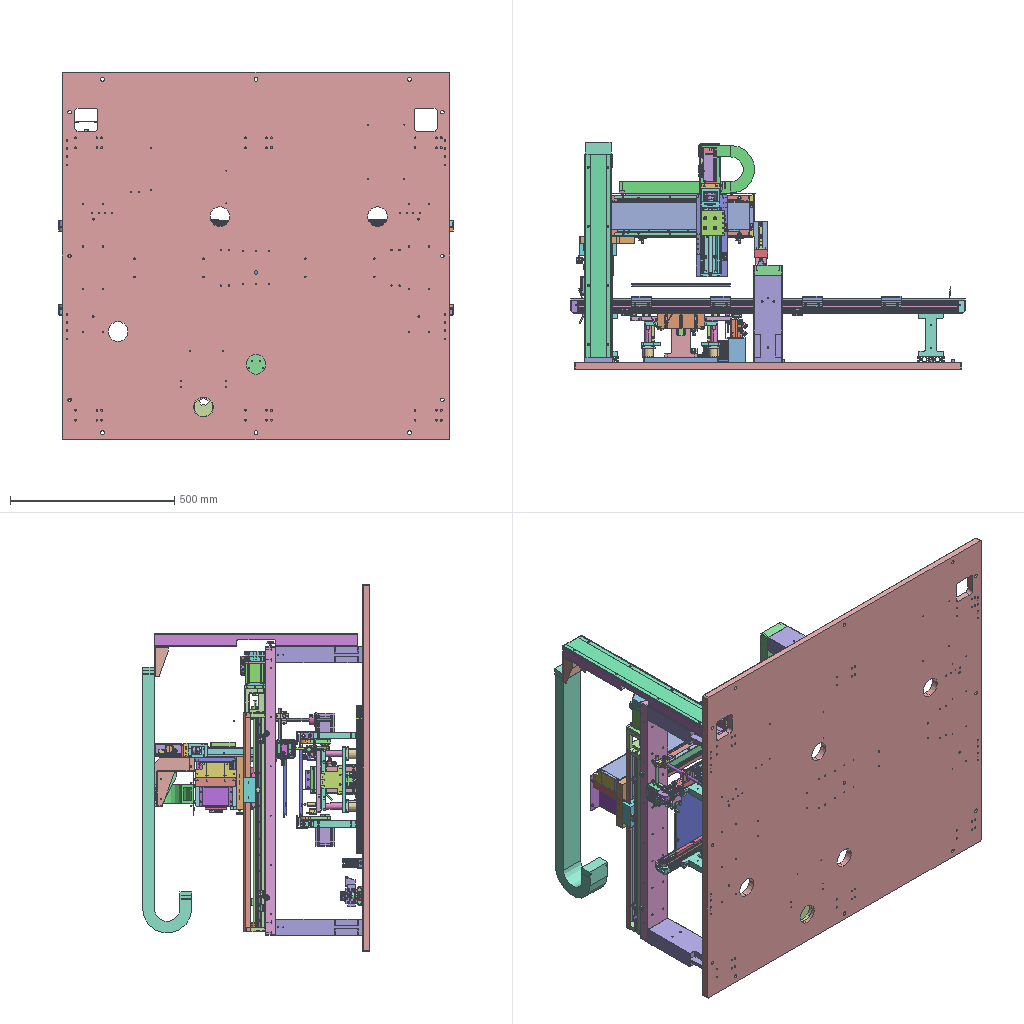Assembly | STEP file | 141 different items | 353 placed | box 1201 x 691 x 1120 mm
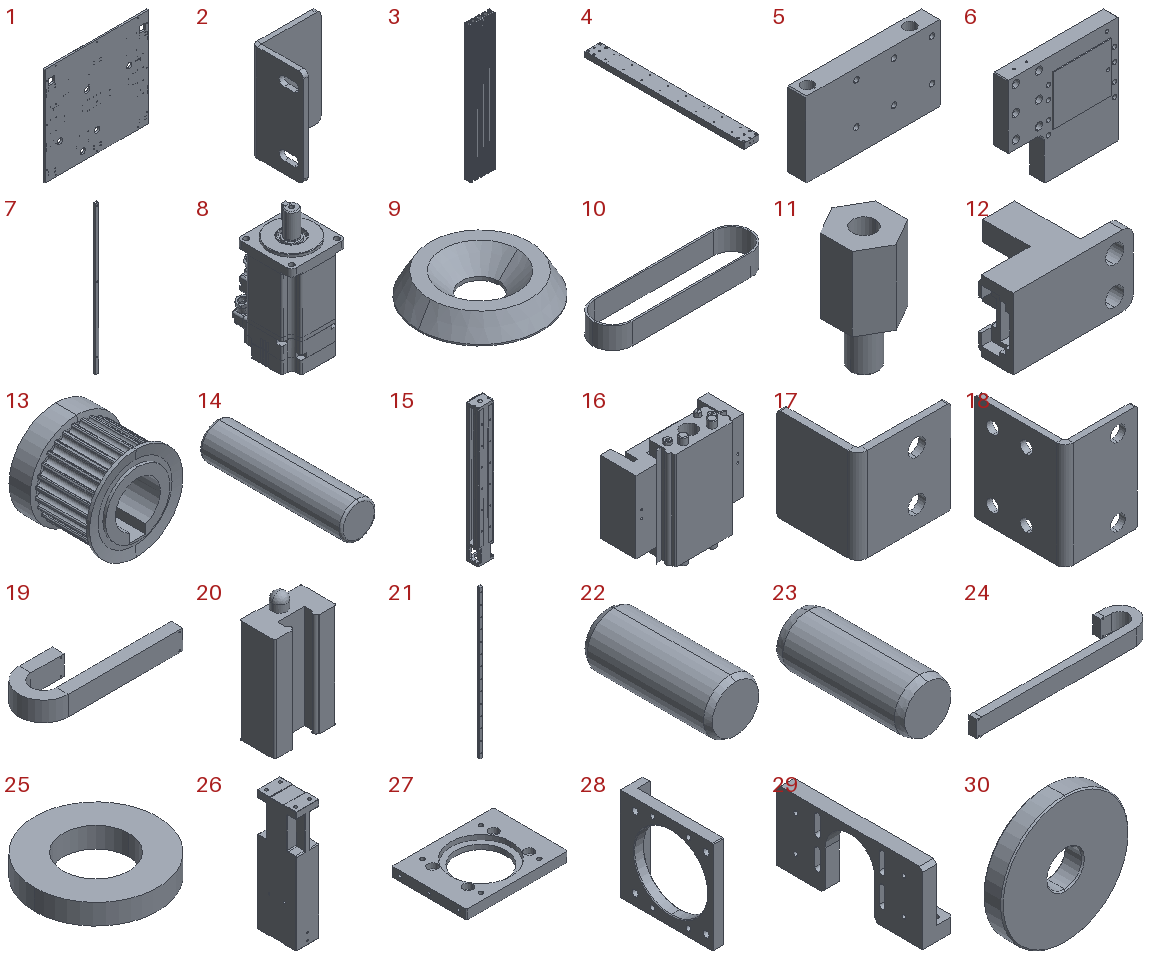Parts list (item | name | quantity | parent item | size | volume):
1 | - | x1 | - | 1180 x 20 x 1120 mm | 25848378 mm3
2 | - | x8 | - | 40 x 32 x 60 mm | 11873 mm3
3 | - | x2 | - | 80 x 20 x 450 mm | 285377 mm3
4 | - | x1 | - | 86 x 880 x 30 mm | 2237479 mm3
5 | - | x1 | - | 125 x 17 x 70 mm | 135841 mm3
6 | - | x1 | - | 167 x 23.5 x 162 mm | 506457 mm3
7 | - | x1 | - | 8 x 5 x 355 mm | 6491 mm3
8 | Servo motor MS1H4-40B30CB-A331Z | x2 | - | - | -
9 | Stainless steel conical countersunk washer M5 | x2 | - | 18 x 18 x 3.2 mm | 517.188 mm3
10 | Timing belt 261-3M-15mm wide_28-28 | x1 | - | 117.86 x 29.16 x 16 mm | 5218 mm3
11 | Brass standoff M3-6x8 | x6 | - | 6 x 6.928 x 13 mm | 251.442 mm3
12 | Photoelectric sensor PM-Y65 | x6 | - | 22.7 x 14.9 x 13.4 mm | 1660 mm3
13 | - | x1 | - | 29 x 26.5 x 29 mm | 9355 mm3
14 | - | x8 | - | 5 x 20 x 5 mm | 392.109 mm3
15 | Single-axis module KK86D20C-640A1 rail | x1 | in Single-axis module KK86D20C-640A1-F0CS0 | 91 x 66.1 x 740 mm | 1447493 mm3
16 | Single-axis module KK8620C slider | x1 | in Single-axis module KK86D20C-640A1-F0CS0 | 112 x 52 x 116 mm | 327270 mm3
17 | Single-axis module KK photoelectric shield | x1 | in Single-axis module KK86D20C-640A1-F0CS0 | 15 x 13 x 15 mm | 422.631 mm3
18 | - | x6 | in Single-axis module KK86D20C-640A1-F0CS0 | 15 x 18.7 x 22 mm | 803.602 mm3
19 | Quiet two-side-openable cable carrier JFLO25x38-R55-25 links | x1 | - | 412 x 145 x 58 mm | 657351 mm3
20 | Slider 15_THK_SSR15XW | x4 | in Rail SSR15XW2SSC1+830LY, 38 | 34 x 19.5 x 65 mm | 30926 mm3
21 | 1 Rail SSR15XW2SSC1+830LY | x1 | in Rail SSR15XW2SSC1+830LY | 15 x 12.5 x 830 mm | 144164 mm3
22 | - | x12 | - | 5 x 12 x 5 mm | 233.269 mm3
23 | Cylindrical pin 4x10-C1 | x6 | - | 4 x 10 x 4 mm | 124.365 mm3
24 | Cable carrier 25x57x1000-R55-quiet-two-side-openable_cable carrier 2 | x1 | - | 810 x 150 x 78 mm | 2572338 mm3
25 | JAZDQ-D30-d16-T5 polyurethane washer | x11 | - | 30 x 30 x 5 mm | 2529 mm3
26 | - | x4 | - | 50 x 86 x 266 mm | 1023683 mm3
27 | - | x1 | - | 86 x 63.5 x 8 mm | 28261 mm3
28 | - | x1 | - | 16 x 65 x 65 mm | 17444 mm3
29 | - | x1 | - | 26 x 124 x 60 mm | 67502 mm3
30 | - | x1 | - | 20 x 3 x 20 mm | 867.998 mm3
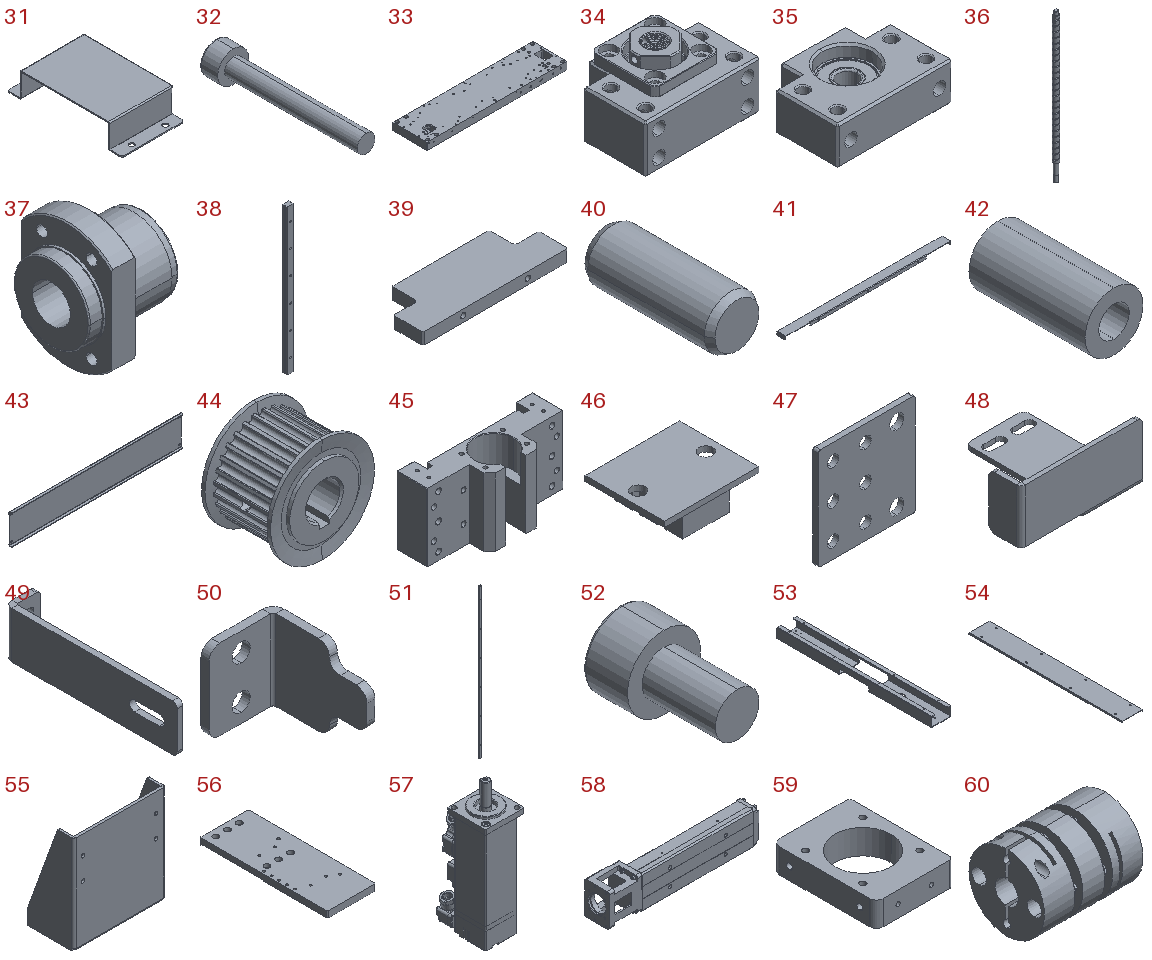31 | - | x1 | - | 57 x 102 x 22 mm | 9559 mm3
32 | M4 socket head cap screw simplified_M4X30 | x3 | - | 7 x 34 x 7 mm | 513.868 mm3
33 | - | x1 | - | 504 x 124 x 26 mm | 1554634 mm3
34 | Screw support seat BK12 | x1 | - | 60 x 43 x 35 mm | 48236 mm3
35 | Screw support seat BF12 | x1 | - | 60 x 43 x 20 mm | 33949 mm3
36 | Screw rod BLK1616-3.6G0+472 | x1 | in Screw rod BLK1616-3.6G0+472LC5 | 16 x 16 x 472 mm | 82941 mm3
37 | Screw nut BLK1616-3.6G | x1 | in Screw rod BLK1616-3.6G0+472LC5 | 38 x 38 x 53 mm | 32346 mm3
38 | Rail SSR15XW1SSC1+370LY | x2 | in 38 | 15 x 12.5 x 370 mm | 64350 mm3
39 | - | x2 | - | 124 x 47 x 10 mm | 44873 mm3
40 | - | x6 | - | 4 x 10 x 4 mm | 123.869 mm3
41 | - | x2 | - | 483 x 25 x 10 mm | 15373 mm3
42 | - | x4 | - | 8 x 16 x 8 mm | 582.577 mm3
43 | - | x1 | - | 504 x 8.5 x 87 mm | 75239 mm3
44 | - | x1 | - | 30 x 21 x 30 mm | 8430 mm3
45 | - | x1 | - | 120 x 45 x 60 mm | 150732 mm3
46 | LJ-sensor2 circuit board V1.0 | x3 | - | 26.5 x 22.2 x 8.5 mm | 1722 mm3
47 | - | x2 | - | 21 x 1.2 x 22 mm | 500.685 mm3
48 | - | x1 | - | 42 x 41 x 20 mm | 2562 mm3
49 | - | x1 | - | 13 x 74 x 20 mm | 3931 mm3
50 | - | x1 | - | 13.5 x 19 x 15 mm | 569.041 mm3
51 | - | x1 | - | 8 x 5 x 590 mm | 11867 mm3
52 | M6 socket head cap screw simplified_M6X10 | x2 | - | 10 x 16 x 10 mm | 685.808 mm3
53 | - | x1 | - | 80 x 620 x 40 mm | 194874 mm3
54 | - | x1 | - | 83 x 620 x 6 mm | 57149 mm3
55 | - | x1 | - | 84 x 42 x 90 mm | 31200 mm3
56 | - | x1 | - | 94 x 250 x 12 mm | 257525 mm3
57 | Servo motor MS1H1-10B30CB-A332Z | x1 | - | - | -
58 | Single-axis module KM3305A+200N0-013LCB | x1 | - | 270 x 44.5 x 64.6 mm | 342909 mm3
59 | - | x1 | - | 43.7 x 59 x 14 mm | 23699 mm3
60 | Double diaphragm coupling LC-A-020DA-06B-08B | x1 | - | 34 x 26 x 26 mm | 11838 mm3
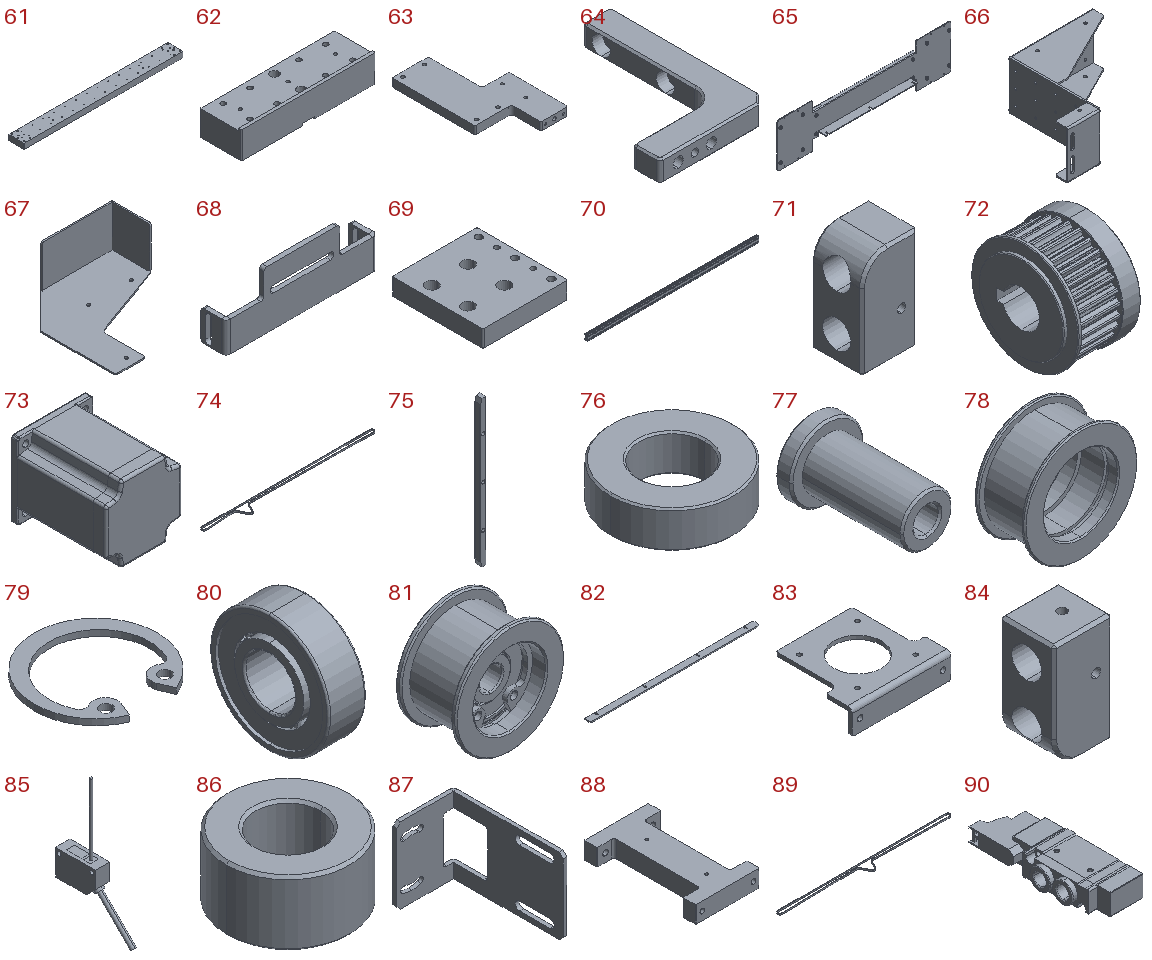61 | - | x1 | - | 880 x 86 x 30 mm | 2237811 mm3
62 | - | x1 | - | 130 x 40 x 26 mm | 113465 mm3
63 | - | x1 | - | 94 x 168 x 12 mm | 120953 mm3
64 | - | x1 | - | 59 x 86 x 12 mm | 20326 mm3
65 | - | x1 | - | 520 x 33 x 132 mm | 111662 mm3
66 | - | x1 | - | 145 x 115 x 60 mm | 47899 mm3
67 | - | x1 | - | 150 x 155 x 60 mm | 44145 mm3
68 | - | x1 | - | 100 x 16.5 x 38 mm | 9262 mm3
69 | - | x1 | - | 70 x 75 x 14 mm | 67812 mm3
70 | - | x2 | - | 1157 x 20 x 40 mm | 344768 mm3
71 | - | x2 | - | 21.5 x 20 x 40 mm | 13498 mm3
72 | - | x2 | - | 19.5 x 29 x 29 mm | 9304 mm3
73 | PN_0001 stepper motor 24HS8404-10PJ3 | x2 | - | 60 x 96 x 60 mm | 237550 mm3
74 | Timing belt 2505-S3M-10mm wide | x2 | - | 1199 x 90.84 x 10 mm | 50146 mm3
75 | - | x6 | - | 13.5 x 14 x 349 mm | 58115 mm3
76 | - | x4 | - | 15 x 15 x 4.5 mm | 566.131 mm3
77 | - | x4 | - | 11.5 x 18.1 x 11.5 mm | 810.877 mm3
78 | - | x4 | - | 29 x 13 x 29 mm | 3455 mm3
79 | Hole-type circlip A-type 19 | x4 | - | 20.5 x 19.72 x 1 mm | 114.602 mm3
80 | Deep groove ball bearing 698ZZ | x4 | - | 6 x 19 x 19 mm | 925.778 mm3
81 | Flange idler ENG11-D20-T11 | x4 | - | 24 x 13.4 x 24 mm | 3034 mm3
82 | - | x4 | - | 600 x 23 x 4 mm | 54278 mm3
83 | - | x2 | - | 80 x 71 x 20 mm | 14540 mm3
84 | - | x2 | - | 21.5 x 20 x 40 mm | 13489 mm3
85 | Small photoelectric sensor CX-441 | x3 | - | 11.2 x 58.715 x 100.215 mm | 7246 mm3
86 | - | x4 | - | 9.5 x 9.5 x 5 mm | 254.414 mm3
87 | - | x2 | - | 32 x 60 x 40 mm | 5405 mm3
88 | - | x4 | - | 75 x 131 x 20 mm | 113693 mm3
89 | - | x2 | - | 1201 x 92.285 x 10 mm | 50245 mm3
90 | Solenoid valve 7V110-06-B terminal type cable length 0.5m | x5 | - | 32.5 x 92.3 x 16.6 mm | 31794 mm3
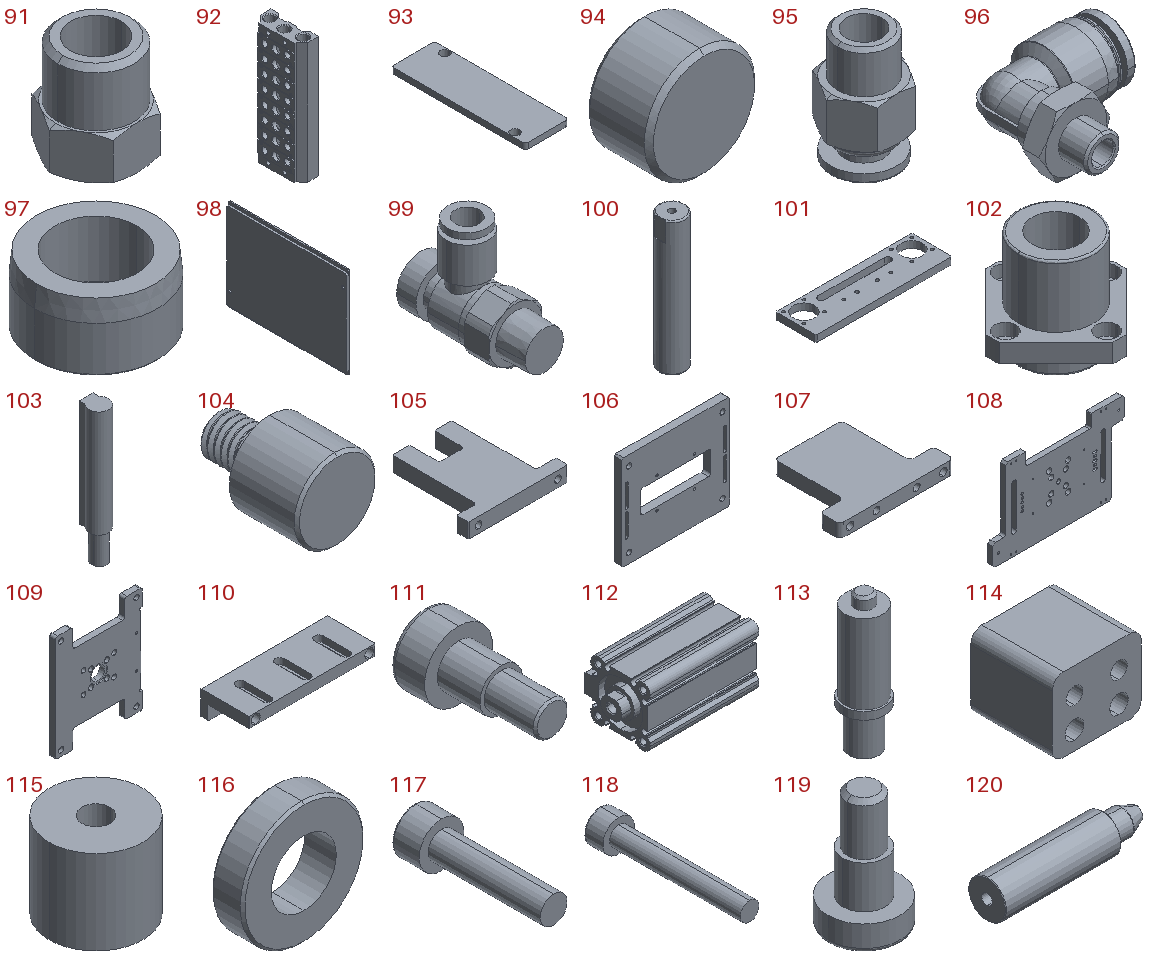91 | Silencer BSLM02_APC6-02 | x4 | - | 16.166 x 14 x 16.962 mm | 1893 mm3
92 | Solenoid valve base 7V100M8F | x1 | - | 22.8 x 57.5 x 146 mm | 85064 mm3
93 | Blind plate 7V100M | x3 | - | 15 x 46.5 x 2 mm | 1363 mm3
94 | 1-4 plug | x1 | - | 12 x 6.95 x 12 mm | 518.038 mm3
95 | Threaded straight fitting APC6-01 | x10 | - | 13.856 x 12 x 20.5 mm | 1319 mm3
96 | Pipe fitting PL1001 | x1 | - | 35.315 x 34 x 18 mm | 5648 mm3
97 | - | x2 | - | 12 x 12 x 6.5 mm | 386.592 mm3
98 | - | x2 | - | 8 x 300 x 230 mm | 529041 mm3
99 | Speed control valve AS2201F-01-06SA | x2 | - | 13 x 30.6 x 26.1 mm | 3953 mm3
100 | - | x4 | - | 20 x 20 x 103 mm | 31531 mm3
101 | - | x2 | - | 202 x 60 x 10 mm | 92729 mm3
102 | Flanged linear bearing LMJ11-D20 | x4 | - | 54 x 54 x 42 mm | 26412 mm3
103 | Solid-state magnetic switch D-M9N | x2 | - | 4 x 4.6 x 28 mm | 365.402 mm3
104 | - | x8 | - | 6 x 8.8 x 6 mm | 161.192 mm3
105 | - | x2 | - | 100 x 97 x 15 mm | 82141 mm3
106 | - | x1 | - | 230 x 16 x 202 mm | 593359 mm3
107 | - | x2 | - | 85 x 66.5 x 10 mm | 36549 mm3
108 | - | x1 | - | 310 x 12 x 200 mm | 529543 mm3
109 | - | x1 | - | 185 x 12 x 225 mm | 366381 mm3
110 | - | x1 | - | 145 x 55 x 28 mm | 101226 mm3
111 | External thread shoulder bolt MSB10-10 | x1 | - | 16 x 30 x 16 mm | 2915 mm3
112 | Slim cylinder CDQ2A32-50DZ_with magnet | x1 | - | 90 x 49.5 x 45 mm | 103379 mm3
113 | - | x8 | - | 5.5 x 5.5 x 18 mm | 266.671 mm3
114 | - | x4 | - | 24 x 22 x 20 mm | 7795 mm3
115 | - | x2 | - | 10 x 10 x 9 mm | 537.212 mm3
116 | - | x1 | - | 15.5 x 4 x 15.5 mm | 539.201 mm3
117 | M6 socket head cap screw simplified_M6x25 | x1 | - | 10 x 31 x 10 mm | 1110 mm3
118 | M5 socket head cap screw simplified_M5X35 | x3 | - | 8.5 x 40 x 8.5 mm | 934.046 mm3
119 | - | x3 | - | 8.5 x 8.5 x 14 mm | 317.59 mm3
120 | - | x1 | - | 48 x 12 x 12 mm | 4513 mm3
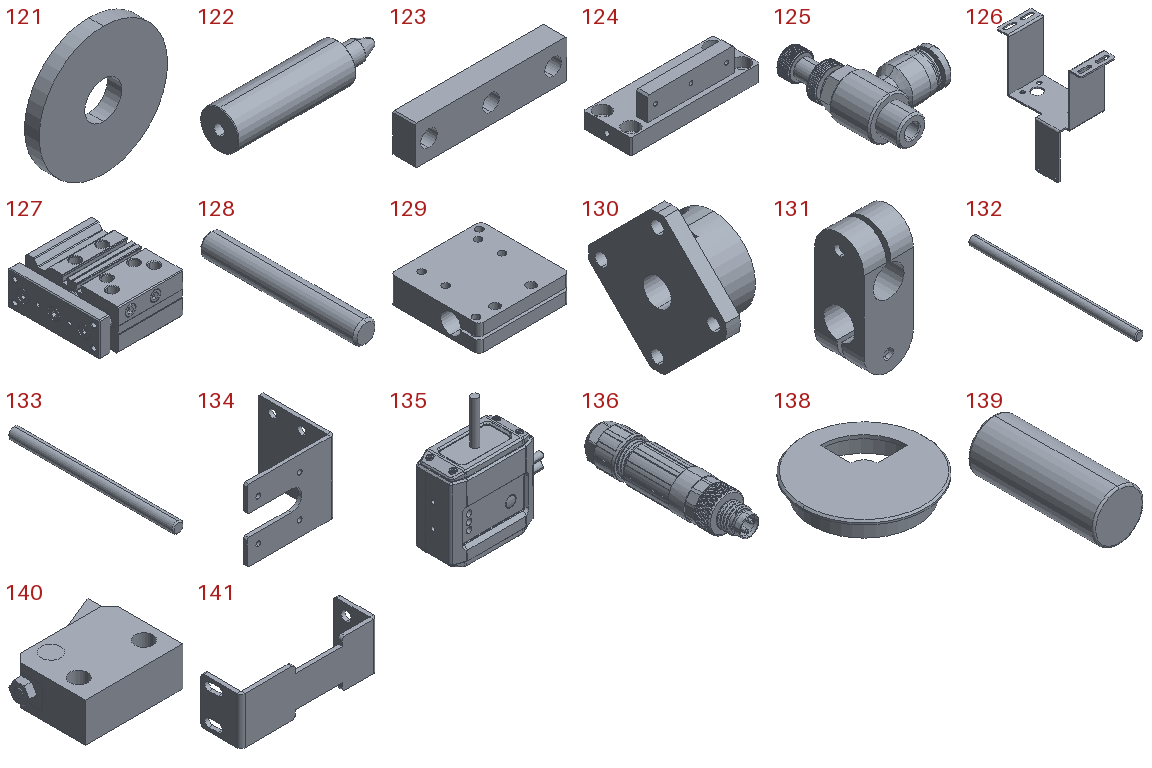121 | - | x1 | - | 35 x 4 x 35 mm | 3528 mm3
122 | - | x1 | - | 48 x 12 x 12 mm | 4302 mm3
123 | - | x1 | - | 55 x 8 x 14 mm | 5679 mm3
124 | - | x1 | - | 82 x 30 x 25 mm | 27843 mm3
125 | Exhaust throttle valve PSL601A | x2 | - | 30.2 x 41.6 x 14.2 mm | 4827 mm3
126 | - | x1 | - | 60 x 122 x 139 mm | 30068 mm3
127 | Three-axis cylinder TCM-20x20-S | x1 | - | 73 x 83 x 36 mm | 154063 mm3
128 | - | x1 | - | 10 x 70 x 10 mm | 5468 mm3
129 | - | x1 | - | 45 x 44 x 13 mm | 20538 mm3
130 | Guide shaft support STHWS10 | x1 | - | 20 x 49 x 49 mm | 14722 mm3
131 | Ultra-simple post clamp ALKW10 | x2 | - | 16 x 16 x 39 mm | 6075 mm3
132 | - | x1 | - | 10 x 190 x 10 mm | 14893 mm3
133 | - | x1 | - | 10 x 150 x 10 mm | 11752 mm3
134 | - | x1 | - | 60 x 50 x 49 mm | 11507 mm3
135 | Code reader ICW74ES-HR | x1 | - | - | -
136 | Plug (straight male) | x16 | - | - | -
137 | I/O junction box 23N8S1 | x2 | - | - | -
138 | - | x1 | - | 70 x 70 x 12 mm | 8548 mm3
139 | - | x16 | - | 8 x 20 x 8 mm | 1004 mm3
140 | Check valve assembly ATBJ7SA-S-BL | x2 | - | 32.5 x 29 x 12 mm | 7437 mm3
141 | - | x2 | - | 87 x 25.5 x 30 mm | 8708 mm3
Placements (level | parent | child | x y z in mm | rotation matrix by rows), first 283 of 370 lines:
1 | subassembly 2 | subassembly 3 | -0.0 -0.0 -0.0 | 1 0 0 0 1 0 0 0 1
1 | subassembly 2 | subassembly 4 | -175.0 190.0 111.5 | 0 0 1 0 1 0 -1 0 -0
1 | subassembly 2 | subassembly 4 | -115.0 190.0 -183.5 | 0 0 -1 0 1 0 1 0 0
1 | subassembly 2 | subassembly 4 | 405.0 190.0 -183.5 | 0 0 -1 0 1 0 1 0 0
1 | subassembly 2 | subassembly 4 | 345.0 190.0 111.5 | 0 0 1 0 1 0 -1 0 -0
1 | subassembly 2 | subassembly 4 | 105.0 190.0 111.5 | 0 0 1 0 1 0 -1 0 -0
1 | subassembly 2 | subassembly 4 | 165.0 190.0 -183.5 | 0 0 -1 0 1 0 1 0 0
1 | subassembly 2 | subassembly 4 | -415.0 190.0 111.5 | 0 0 1 0 1 0 -1 0 -0
1 | subassembly 2 | subassembly 4 | -355.0 190.0 -183.5 | 0 0 -1 0 1 0 1 0 0
1 | subassembly 2 | subassembly 5 | -526.0 30.0 -36.0 | 1 0 0 0 1 0 0 0 1
1 | subassembly 2 | subassembly 5 | 466.0 30.0 -36.0 | 1 0 0 0 1 0 0 0 1
1 | subassembly 2 | subassembly 6 | -207.203 113.811 -80.031 | 1 0 0 0 1 0 0 0 1
2 | subassembly 6 | subassembly 7 | -309.797 172.189 10.031 | 1 0 0 0 0 1 0 -1 -0
2 | subassembly 6 | subassembly 8 | -292.297 309.189 23.923 | 1 0 0 0 -1 0 0 0 -1
2 | subassembly 6 | subassembly 9 | -309.797 270.189 50.923 | -1 0 0 0 1 0 0 0 -1
2 | subassembly 6 | subassembly 10 | -17.797 291.389 44.923 | 0 0 1 0 -1 0 1 0 0
2 | subassembly 6 | Servo motor MS1H4-40B30CB-A331Z | -309.797 234.189 330.031 | -1 0 0 0 1 0 0 0 -1
2 | subassembly 6 | Stainless steel conical countersunk washer M5 | -354.397 198.689 -314.969 | 0 0 -1 0 1 0 1 0 -0
2 | subassembly 6 | Timing belt 261-3M-15mm wide_28-28 | -320.297 354.189 78.123 | 0 0 -1 0 -1 0 -1 0 -0
2 | subassembly 6 | Brass standoff M3-6x8 | -237.797 281.189 -41.077 | -0.9237 -0.383 0 -0.383 0.9237 0 0 0 -1
2 | subassembly 6 | Brass standoff M3-6x8 | -218.797 281.189 -41.077 | -0.9237 -0.383 0 -0.383 0.9237 0 0 0 -1
2 | subassembly 6 | Stainless steel conical countersunk washer M5 | -354.397 198.689 185.031 | 0 0 -1 0 1 0 1 0 -0
2 | subassembly 6 | Photoelectric sensor PM-Y65 | -371.297 224.289 -303.969 | 0 0 1 0 1 0 -1 0 -0
2 | subassembly 6 | Photoelectric sensor PM-Y65 | -371.297 224.289 166.031 | 0 0 1 0 1 0 -1 0 -0
2 | subassembly 6 | Brass standoff M3-6x8 | -300.297 187.189 445.031 | -1 0 0 0 -1 0 0 0 1
2 | subassembly 6 | Brass standoff M3-6x8 | -319.297 187.189 445.031 | -1 0 0 0 -1 0 0 0 1
2 | subassembly 6 | Photoelectric sensor PM-Y65 | 121.203 273.089 58.223 | 1 0 0 0 -1 0 0 0 -1
2 | subassembly 6 | Photoelectric sensor PM-Y65 | -173.797 273.089 58.223 | 1 0 0 0 -1 0 0 0 -1
2 | subassembly 6 | Servo motor MS1H4-40B30CB-A331Z | -299.997 354.189 -10.577 | 0 0 -1 1 0 0 0 -1 -0
2 | subassembly 6 | subassembly 11 | -319.797 354.189 -10.577 | 0 1 0 0.3098 0 -0.9508 -0.9508 0 -0.3098
2 | subassembly 6 | subassembly 12 | -309.797 170.988 -420.969 | 0.6062 0 -0.7953 0 1 0 0.7953 0 0.6062
2 | subassembly 6 | subassembly 12 | -309.797 170.988 -388.969 | -0.2227 0 -0.9749 0 1 0 0.9749 0 -0.2227
2 | subassembly 6 | subassembly 12 | -309.797 170.988 409.031 | -0.9033 0 0.429 0 1 0 -0.429 0 -0.9033
2 | subassembly 6 | subassembly 12 | -309.797 170.988 441.031 | -0.00379 0 -1 0 1 0 1 0 -0.00379
2 | subassembly 6 | Single-axis module KK86D20C-640A1-F0CS0 | -303.659 213.204 235.031 | -1 0 0 0 1 0 0 0 -1
3 | Single-axis module KK86D20C-640A1-F0CS0 | Single-axis module KK86D20C-640A1 rail | 6.139 -1.115 -0.0 | 1 0 0 0 1 0 0 0 1
3 | Single-axis module KK86D20C-640A1-F0CS0 | Single-axis module KK8620C slider | 6.139 -1.115 121.307 | 1 0 0 0 1 0 0 0 1
3 | Single-axis module KK86D20C-640A1-F0CS0 | Single-axis module KK photoelectric shield | 65.639 19.985 222.107 | -1 0 0 0 -1 0 0 0 1
3 | Single-axis module KK86D20C-640A1-F0CS0 | subassembly 13 | 53.139 -3.015 63.133 | 0 1 0 1 0 0 0 0 -1
3 | Single-axis module KK86D20C-640A1-F0CS0 | subassembly 13 | 53.139 -3.015 582.456 | 0 1 0 1 0 0 0 0 -1
2 | subassembly 6 | Quiet two-side-openable cable carrier JFLO25x38-R55-25 links | -3.797 495.689 0.4234 | -1 0 0 0 1 0 0 0 -1
2 | subassembly 6 | subassembly 12 | 207.203 173.189 409.031 | -0.00379 0 -1 0 1 0 1 0 -0.00379
2 | subassembly 6 | subassembly 12 | 207.203 173.189 441.031 | -0.00379 0 -1 0 1 0 1 0 -0.00379
2 | subassembly 6 | subassembly 12 | 207.203 173.189 -388.969 | -0.00379 0 -1 0 1 0 1 0 -0.00379
2 | subassembly 6 | subassembly 12 | 207.203 173.189 -420.969 | -0.00379 0 -1 0 1 0 1 0 -0.00379
2 | subassembly 6 | Rail SSR15XW2SSC1+830LY | 185.703 214.689 10.031 | 1 0 0 0 1 0 0 0 1
3 | Rail SSR15XW2SSC1+830LY | Slider 15_THK_SSR15XW | 0.0 0.0 -119.107 | 1 0 0 0 1 0 0 0 1
3 | Rail SSR15XW2SSC1+830LY | Slider 15_THK_SSR15XW | 0.0 0.0 134.893 | -1 0 0 0 1 0 0 0 -1
3 | Rail SSR15XW2SSC1+830LY | 1 Rail SSR15XW2SSC1+830LY | -0.0 -0.0 -0.0 | 1 0 0 0 1 0 0 0 1
2 | subassembly 6 | subassembly 14 | 195.703 205.189 260.031 | 0.9377 0 -0.3474 0 1 0 0.3474 0 0.9377
2 | subassembly 6 | subassembly 14 | 195.703 205.189 -239.969 | 0.9377 0 -0.3474 0 1 0 0.3474 0 0.9377
2 | subassembly 6 | Cylindrical pin 4x10-C1 | 185.703 249.189 63.923 | 1 0 0 0 1 0 0 0 1
2 | subassembly 6 | Cylindrical pin 4x10-C1 | 185.703 247.189 17.923 | 1 0 0 0 1 0 0 0 1
2 | subassembly 6 | subassembly 14 | 63.555 339.189 117.423 | 1 0 0 0 0 -1 0 1 0
2 | subassembly 6 | subassembly 14 | 63.555 219.189 117.423 | 1 0 0 0 0 -1 0 1 0
2 | subassembly 6 | Cable carrier 25x57x1000-R55-quiet-two-side-openable_cable carrier 2 | -309.797 577.189 -297.469 | 0 0 -1 0 -1 0 -1 0 0
2 | subassembly 6 | JAZDQ-D30-d16-T5 polyurethane washer | 119.203 354.189 74.923 | 0 0 1 -0.933 -0.3598 0 0.3598 -0.933 -0
2 | subassembly 6 | JAZDQ-D30-d16-T5 polyurethane washer | 114.203 354.189 74.923 | 0 0 1 -0.933 -0.3598 0 0.3598 -0.933 -0
2 | subassembly 6 | JAZDQ-D30-d16-T5 polyurethane washer | 109.203 354.189 74.923 | 0 0 1 -0.933 -0.3598 0 0.3598 -0.933 -0
2 | subassembly 6 | Cylindrical pin 4x10-C1 | -1.945 298.189 222.423 | 0 1 0 0 0 1 1 0 0
2 | subassembly 6 | Cylindrical pin 4x10-C1 | -1.945 238.189 222.423 | 0 1 0 0 0 1 1 0 0
2 | subassembly 6 | Cylindrical pin 4x10-C1 | -5.945 283.189 110.423 | -1 0 0 0 0 1 0 1 0
2 | subassembly 6 | Cylindrical pin 4x10-C1 | -5.945 253.189 110.423 | -1 0 0 0 0 1 0 1 0
2 | subassembly 6 | subassembly 15 | -309.797 172.189 -404.969 | 0 1 0 0 0 -1 -1 0 0
2 | subassembly 6 | subassembly 15 | -309.797 172.189 425.031 | 0 -1 0 0 0 -1 1 0 -0
2 | subassembly 6 | subassembly 16 | -309.797 234.939 326.031 | 1 0 0 0 1 0 0 0 1
2 | subassembly 6 | subassembly 17 | -299.997 354.189 -13.077 | -1 0 0 0 0 -1 0 -1 -0
2 | subassembly 6 | subassembly 18 | -312.997 354.189 -6.077 | 1 0 0 0 -1 0 0 0 -1
2 | subassembly 6 | subassembly 19 | -332.997 354.189 -10.577 | 0 1 0 -1 0 0 0 0 1
2 | subassembly 6 | subassembly 20 | -340.997 354.189 -7.577 | 0 0 -1 0 -1 0 -1 0 -0
2 | subassembly 6 | subassembly 13 | -356.797 210.189 -303.969 | 0 -1 0 1 0 0 0 0 1
2 | subassembly 6 | subassembly 21 | 0.1459 311.218 -469.077 | -1 0 0 0 -1 0 0 0 1
3 | subassembly 21 | M4 socket head cap screw simplified_M4X30 | 254.943 -13.471 529.0 | -0.6464 0 0.763 0.763 0 0.6464 0 1 -0
3 | subassembly 21 | M4 socket head cap screw simplified_M4X30 | -122.057 -15.971 529.0 | -0.9254 0 0.3791 0.3791 0 0.9254 0 1 0
3 | subassembly 21 | subassembly 22 | 90.443 -42.971 493.0 | 1 0 0 0 1 0 0 0 1
3 | subassembly 21 | Screw support seat BK12 | 286.443 -42.971 519.0 | 0 0 1 1 0 0 0 1 -0
3 | subassembly 21 | Screw support seat BF12 | -136.557 -42.971 519.0 | 0 0 1 1 0 0 0 1 -0
3 | subassembly 21 | Screw rod BLK1616-3.6G0+472LC5 | 228.501 -28.195 524.837 | -1 0 0 0 0 -1 0 -1 -0
4 | Screw rod BLK1616-3.6G0+472LC5 | Screw rod BLK1616-3.6G0+472 | -44.942 -19.163 14.776 | 0 0 1 -1 0 0 0 -1 0
4 | Screw rod BLK1616-3.6G0+472LC5 | Screw nut BLK1616-3.6G | 248.91 -19.163 14.776 | 1 0 0 0 1 0 0 0 1
3 | subassembly 21 | Rail SSR15XW1SSC1+370LY | 65.943 -83.971 531.5 | 0 0 1 1 0 0 0 1 -0
4 | Rail SSR15XW1SSC1+370LY | Rail SSR15XW1SSC1+370LY | 0.0 0.0 0.0 | 1 0 0 0 1 0 0 0 1
4 | Rail SSR15XW1SSC1+370LY | Slider 15_THK_SSR15XW | -0.0 -0.0 -258.353 | 1 0 0 0 1 0 0 0 1
3 | subassembly 21 | subassembly 23 | -156.557 -42.971 542.5 | 0 0 -1 -1 0 0 0 1 0
3 | subassembly 21 | JAZDQ-D30-d16-T5 polyurethane washer | -124.057 -42.971 544.0 | 0 0 -1 0.2217 -0.9751 0 -0.9751 -0.2217 0
3 | subassembly 21 | M4 socket head cap screw simplified_M4X30 | 254.943 -72.471 529.0 | 0.406 0 0.9139 0.9139 0 -0.406 0 1 -0
3 | subassembly 21 | subassembly 24 | 232.443 -74.471 512.5 | 0.9991 0 -0.04147 0.04147 0 0.9991 0 -1 0
3 | subassembly 21 | subassembly 24 | -101.557 -11.471 512.5 | 0.9991 0 -0.04147 0.04147 0 0.9991 0 -1 0
3 | subassembly 21 | subassembly 25 | 90.443 19.029 531.5 | -1 0 0 0 0 1 0 1 -0
3 | subassembly 21 | subassembly 26 | -122.057 -72.471 509.0 | 1 0 0 0 0 -1 0 1 0
3 | subassembly 21 | subassembly 27 | 90.443 0.5293 567.5 | 1 0 0 0 0 -1 0 1 -0
3 | subassembly 21 | subassembly 28 | 319.943 -42.971 544.0 | 0 1 0 -1 0 0 0 0 1
3 | subassembly 21 | subassembly 29 | -28.91 -42.971 557.0 | 0 0 1 1 0 0 0 1 0
3 | subassembly 21 | subassembly 26 | 254.943 -72.471 519.0 | 1 0 0 0 0 -1 0 1 -0
3 | subassembly 21 | subassembly 24 | 65.443 -74.471 512.5 | 0.9991 0 -0.04147 0.04147 0 0.9991 0 -1 0
3 | subassembly 21 | subassembly 26 | -122.057 -15.971 519.0 | 1 0 0 0 0 -1 0 1 0
3 | subassembly 21 | JAZDQ-D30-d16-T5 polyurethane washer | 271.443 -42.971 544.0 | 0 0 -1 0.2976 0.9547 0 0.9547 -0.2976 0
3 | subassembly 21 | subassembly 26 | 254.943 -13.471 519.0 | 1 0 0 0 0 -1 0 1 -0
3 | subassembly 21 | subassembly 23 | 337.443 -42.971 542.5 | 0 0 1 1 0 0 0 1 -0
3 | subassembly 21 | subassembly 25 | 90.443 -104.971 531.5 | 1 0 0 0 0 -1 0 1 -0
3 | subassembly 21 | Rail SSR15XW1SSC1+370LY | 65.943 -1.971 531.5 | 0 0 1 1 0 0 0 1 -0
4 | Rail SSR15XW1SSC1+370LY | Rail SSR15XW1SSC1+370LY | 0.0 0.0 0.0 | 1 0 0 0 1 0 0 0 1
4 | Rail SSR15XW1SSC1+370LY | Slider 15_THK_SSR15XW | -0.0 -0.0 -258.353 | 1 0 0 0 1 0 0 0 1
3 | subassembly 21 | subassembly 24 | 65.443 -11.471 512.5 | 0.9991 0 -0.04147 0.04147 0 0.9991 0 -1 0
3 | subassembly 21 | subassembly 24 | -101.557 -74.471 512.5 | 0.9991 0 -0.04147 0.04147 0 0.9991 0 -1 0
3 | subassembly 21 | subassembly 24 | 232.443 -11.471 512.5 | 0.9991 0 -0.04147 0.04147 0 0.9991 0 -1 0
2 | subassembly 6 | subassembly 13 | -356.797 210.189 166.031 | 0 -1 0 1 0 0 0 0 1
2 | subassembly 6 | LJ-sensor2 circuit board V1.0 | -228.297 281.189 -55.577 | 1 0 0 0 1 0 0 0 1
2 | subassembly 6 | LJ-sensor2 circuit board V1.0 | -309.797 187.189 459.531 | 1 0 0 0 -1 0 0 0 -1
2 | subassembly 6 | subassembly 30 | 120.703 287.189 61.923 | 0 0 -1 0 -1 0 -1 0 -0
2 | subassembly 6 | subassembly 31 | 59.055 289.189 86.923 | 0 0 -1 0 1 0 1 0 -0
2 | subassembly 6 | subassembly 32 | -253.797 248.189 -327.959 | 1 0 0 0 1 0 0 0 1
2 | subassembly 6 | subassembly 30 | -174.297 287.189 61.923 | 0 0 -1 0 -1 0 -1 0 -0
2 | subassembly 6 | JAZDQ-D30-d16-T5 polyurethane washer | -256.297 354.189 74.923 | 0 0 1 -0.933 -0.3598 0 0.3598 -0.933 -0
2 | subassembly 6 | JAZDQ-D30-d16-T5 polyurethane washer | -266.297 354.189 74.923 | 0 0 1 -0.847 -0.5316 0 0.5316 -0.847 -0
2 | subassembly 6 | JAZDQ-D30-d16-T5 polyurethane washer | -261.297 354.189 74.923 | 0 0 1 -0.847 -0.5316 0 0.5316 -0.847 -0
2 | subassembly 6 | subassembly 15 | 207.203 172.189 -404.969 | 0 -1 0 0 0 -1 1 0 -0
2 | subassembly 6 | subassembly 15 | 207.203 172.189 425.031 | 0 -1 0 0 0 -1 1 0 -0
2 | subassembly 6 | subassembly 33 | 65.055 346.489 144.423 | 1 0 0 0 0 -1 0 1 -0
2 | subassembly 6 | subassembly 34 | -352.997 221.189 -84.969 | 0 -1 0 1 0 0 0 0 1
2 | subassembly 6 | M6 socket head cap screw simplified_M6X10 | 198.203 208.189 -408.969 | 1 0 0 0 1 0 0 0 1
2 | subassembly 6 | M6 socket head cap screw simplified_M6X10 | 198.203 208.189 429.031 | 1 0 0 0 1 0 0 0 1
2 | subassembly 6 | subassembly 35 | -309.797 231.189 452.031 | 1 0 0 0 1 0 0 0 1
2 | subassembly 6 | subassembly 36 | -309.797 231.189 491.031 | -1 0 0 0 -1 0 0 0 1
2 | subassembly 6 | subassembly 37 | -309.797 539.189 450.031 | 1 0 0 0 -1 0 0 0 -1
2 | subassembly 6 | subassembly 38 | 36.055 293.189 99.423 | 1 0 0 0 1 0 0 0 1
2 | subassembly 6 | subassembly 39 | 735.493 -91.478 -19.184 | -1 0 0 0 1 0 0 0 -1
3 | subassembly 39 | Brass standoff M3-6x8 | 679.938 536.666 -143.758 | 0 0 -1 -0.383 0.9237 0 0.9237 0.383 0
3 | subassembly 39 | LJ-sensor2 circuit board V1.0 | 665.438 536.666 -153.258 | 0 0 1 0 1 0 -1 0 -0
3 | subassembly 39 | Servo motor MS1H1-10B30CB-A332Z | 704.438 548.666 -153.258 | 0 1 0 0 0 -1 -1 0 0
3 | subassembly 39 | Photoelectric sensor PM-Y65 | 655.338 409.666 -148.708 | 0 0 1 -1 0 0 0 -1 0
3 | subassembly 39 | Photoelectric sensor PM-Y65 | 655.338 321.666 -148.708 | 0 0 1 -1 0 0 0 -1 0
3 | subassembly 39 | Single-axis module KM3305A+200N0-013LCB | 704.438 529.666 -153.608 | 0 0 1 -1 0 0 0 -1 0
3 | subassembly 39 | Brass standoff M3-6x8 | 679.938 536.666 -162.758 | 0 0 -1 -0.383 0.9237 0 0.9237 0.383 -0
3 | subassembly 39 | subassembly 13 | 669.838 409.666 -134.608 | 0 -1 0 0 0 1 -1 0 -0
3 | subassembly 39 | subassembly 13 | 669.838 321.666 -134.608 | 0 -1 0 0 0 1 -1 0 -0
3 | subassembly 39 | subassembly 40 | 704.438 529.666 -153.258 | 0 -1 0 0 0 1 -1 0 -0
3 | subassembly 39 | Double diaphragm coupling LC-A-020DA-06B-08B | 704.438 512.166 -153.608 | 0 -0.6848 0.7288 -1 0 0 0 -0.7288 -0.6848
2 | subassembly 6 | subassembly 41 | 207.203 202.189 10.031 | 0 1 0 0 0 -1 -1 0 -0
2 | subassembly 6 | subassembly 42 | 185.703 250.189 17.923 | 0 -1 0 0 0 -1 1 0 -0
2 | subassembly 6 | subassembly 43 | 111.703 416.189 17.923 | 1 0 0 0 1 0 0 0 1
2 | subassembly 6 | subassembly 44 | 179.703 250.189 82.923 | 0 0 1 0 1 0 -1 0 0
2 | subassembly 6 | subassembly 45 | -90.297 423.189 -6.077 | -1 0 0 0 1 0 0 0 -1
2 | subassembly 6 | subassembly 46 | 31.555 420.189 111.423 | 0 0 1 0 1 0 -1 0 0
2 | subassembly 6 | subassembly 47 | 1.555 418.189 111.423 | 0 0 1 0 1 0 -1 0 0
2 | subassembly 6 | subassembly 48 | -328.797 292.189 77.923 | 1 0 0 0 1 0 0 0 1
2 | subassembly 6 | JAZDQ-D30-d16-T5 polyurethane washer | -309.797 234.189 -402.469 | -0.9751 -0.2217 0 0.2217 -0.9751 0 0 0 1
2 | subassembly 6 | JAZDQ-D30-d16-T5 polyurethane washer | -309.797 234.189 -397.469 | -0.9751 -0.2217 0 0.2217 -0.9751 0 0 0 1
2 | subassembly 6 | JAZDQ-D30-d16-T5 polyurethane washer | -309.797 234.189 -392.469 | -0.9751 -0.2217 0 0.2217 -0.9751 0 0 0 1
2 | subassembly 6 | subassembly 49 | 41.055 331.489 144.423 | 1 0 0 0 1 0 0 0 1
1 | subassembly 2 | subassembly 50 | 240.815 73.521 1642.428 | 1 0 0 0 1 0 0 0 1
2 | subassembly 50 | subassembly 51 | 337.685 117.479 -1812.928 | -1 0 0 0 0 -1 0 -1 0
2 | subassembly 50 | subassembly 51 | 337.685 117.479 -1543.928 | -1 0 0 0 0 -1 0 -1 0
2 | subassembly 50 | subassembly 52 | 320.685 137.479 -1538.928 | -1 0 0 0 0 -1 0 -1 0
2 | subassembly 50 | subassembly 53 | -224.21 96.281 -1716.546 | 0 -1 0 0 0 -1 1 0 0
2 | subassembly 50 | PN_0001 stepper motor 24HS8404-10PJ3 | -240.815 61.979 -1475.928 | 0 0 -1 1 0 0 0 -1 0
2 | subassembly 50 | Timing belt 2505-S3M-10mm wide | -454.06 107.169 -1800.428 | 1 0 0 0 1 0 0 0 1
2 | subassembly 50 | subassembly 54 | -765.315 127.779 -1795.928 | 0 0 1 -1 0 0 0 -1 -0
2 | subassembly 50 | subassembly 55 | 343.257 123.04 -1576.042 | -0.2643 0 -0.9644 0.9644 0 -0.2643 0 -1 0
3 | subassembly 55 | subassembly 56 | -1.619 -17.614 -0.0 | -0.1925 -0.9813 0 0 0 -1 0.9813 -0.1925 -0
3 | subassembly 55 | subassembly 57 | -1.619 -27.214 -0.0 | -0.7472 0 0.6646 0 1 0 -0.6646 0 -0.7472
3 | subassembly 55 | subassembly 58 | -1.619 -6.614 0.0 | 0.8812 0 -0.4728 0 -1 0 -0.4728 0 -0.8812
3 | subassembly 55 | Hole-type circlip A-type 19 | -1.619 -11.264 -0.0 | 0.797 0.604 0 0 0 1 0.604 -0.797 -0
3 | subassembly 55 | Deep groove ball bearing 698ZZ | -1.619 -14.614 -0.0 | 0 -0.4498 0.8931 1 0 0 0 0.8931 0.4498
2 | subassembly 50 | Flange idler ENG11-D20-T11 | -189.114 107.097 -1585.428 | -0.9999 0 -0.01441 -0.01441 0 0.9999 0 1 -0
2 | subassembly 50 | subassembly 59 | 59.185 141.479 -1805.928 | -1 0 0 0 0 -1 0 -1 0
2 | subassembly 50 | PN_0001 stepper motor 24HS8404-10PJ3 | -240.815 61.979 -1880.928 | 0 0 1 1 0 0 0 1 -0
2 | subassembly 50 | Timing belt 2505-S3M-10mm wide | -454.06 107.169 -1566.428 | 1 0 0 0 1 0 0 0 1
2 | subassembly 50 | subassembly 60 | -240.815 61.979 -1802.928 | -1 0 0 0 -1 0 0 0 1
2 | subassembly 50 | subassembly 60 | -240.815 61.979 -1553.928 | 1 0 0 0 -1 0 0 0 -1
2 | subassembly 50 | subassembly 61 | 320.685 97.479 -1817.928 | -1 0 0 0 0 1 0 1 -0
2 | subassembly 50 | subassembly 61 | -802.315 97.479 -1538.928 | 1 0 0 0 0 1 0 -1 -0
2 | subassembly 50 | Flange idler ENG11-D20-T11 | -188.669 106.648 -1771.428 | -0.0243 0 0.9997 -0.9997 0 -0.0243 0 -1 -0
2 | subassembly 50 | subassembly 52 | -802.315 137.479 -1817.928 | 1 0 0 0 0 -1 0 1 0
2 | subassembly 50 | Flange idler ENG11-D20-T11 | -293.823 106.692 -1585.428 | -0.8165 0 -0.5774 -0.5774 0 0.8165 0 1 0
2 | subassembly 50 | Small photoelectric sensor CX-441 | 309.536 123.145 -1586.328 | 0 0.9945 0.1051 0 -0.1051 0.9945 1 0 -0
2 | subassembly 50 | Flange idler ENG11-D20-T11 | -292.778 106.762 -1771.428 | 0.8859 0 0.4638 -0.4638 0 0.8859 0 -1 -0
2 | subassembly 50 | Small photoelectric sensor CX-441 | -797.949 120.075 -1586.328 | 0 0.9397 -0.342 0 0.342 0.9397 1 0 -0
2 | subassembly 50 | subassembly 59 | 59.185 141.479 -1550.928 | 1 0 0 0 0 -1 0 1 0
2 | subassembly 50 | subassembly 62 | -188.279 107.479 -1558.928 | 0.3759 0.9266 0 -0.9266 0.3759 0 0 0 1
2 | subassembly 50 | subassembly 62 | -293.351 107.479 -1558.928 | 0.3666 0.9304 0 -0.9304 0.3666 0 0 0 1
2 | subassembly 50 | subassembly 53 | -257.42 96.281 -1640.311 | 0 1 0 0 0 -1 -1 0 -0
2 | subassembly 50 | subassembly 62 | -293.351 107.479 -1802.928 | -0.3329 0.943 0 -0.943 -0.3329 0 0 0 1
2 | subassembly 50 | subassembly 62 | -188.279 107.479 -1802.928 | -0.2648 0.9643 0 -0.9643 -0.2648 0 0 0 1
2 | subassembly 50 | subassembly 63 | -790.815 95.479 -1533.928 | 0 0 1 -1 0 0 0 -1 -0
2 | subassembly 50 | subassembly 54 | 283.685 127.779 -1560.928 | 0 0 -1 -1 0 0 0 1 0
2 | subassembly 50 | subassembly 55 | 342.202 122.13 -1780.814 | -0.9157 0 0.4019 0.4019 0 0.9157 0 1 -0
3 | subassembly 55 | subassembly 56 | -1.619 -17.614 -0.0 | -0.8289 -0.5593 0 0 0 -1 0.5593 -0.8289 -0
3 | subassembly 55 | Deep groove ball bearing 698ZZ | -1.619 -14.614 -0.0 | 0 -0.949 0.3152 1 0 0 0 0.3152 0.949
3 | subassembly 55 | subassembly 57 | -1.619 -27.214 -0.0 | -0.06024 0 0.9982 0 1 0 -0.9982 0 -0.06024
3 | subassembly 55 | subassembly 58 | -1.619 -6.614 -0.0 | 0.8812 0 -0.4728 0 -1 0 -0.4728 0 -0.8812
3 | subassembly 55 | Hole-type circlip A-type 19 | -1.619 -11.264 -0.0 | 0.1382 0.9904 0 0 0 1 0.9904 -0.1382 0
2 | subassembly 50 | subassembly 55 | -826.737 122.254 -1576.042 | -0.8782 0 -0.4783 0.4783 0 -0.8782 0 -1 0
3 | subassembly 55 | subassembly 57 | -1.619 -27.214 -0.0 | -0.03997 0 0.9992 0 1 0 -0.9992 0 -0.03997
3 | subassembly 55 | subassembly 58 | -1.619 -6.614 0.0 | 0.8812 0 -0.4728 0 -1 0 -0.4728 0 -0.8812
3 | subassembly 55 | Deep groove ball bearing 698ZZ | -1.619 -14.614 -0.0 | 0 -0.9552 0.2959 1 0 0 0 0.2959 0.9552
3 | subassembly 55 | subassembly 56 | -1.619 -17.614 -0.0 | -0.8401 -0.5424 0 0 0 -1 0.5424 -0.8401 -0
3 | subassembly 55 | Hole-type circlip A-type 19 | -1.619 -11.264 -0.0 | 0.1181 0.993 0 0 0 1 0.993 -0.1181 -0
2 | subassembly 50 | subassembly 55 | -825.662 123.061 -1780.814 | -0.214 0 0.9768 0.9768 0 0.214 0 1 -0
3 | subassembly 55 | subassembly 58 | -1.619 -6.614 -0.0 | 0.8812 0 -0.4728 0 -1 0 -0.4728 0 -0.8812
3 | subassembly 55 | subassembly 57 | -1.619 -27.214 -0.0 | -0.04028 0 0.9992 0 1 0 -0.9992 0 -0.04028
3 | subassembly 55 | Deep groove ball bearing 698ZZ | -1.619 -14.614 0.0 | 0 -0.9551 0.2962 1 0 0 0 0.2962 0.9551
3 | subassembly 55 | subassembly 56 | -1.619 -17.614 -0.0 | -0.84 -0.5426 0 0 0 -1 0.5426 -0.84 -0
3 | subassembly 55 | Hole-type circlip A-type 19 | -1.619 -11.264 0.0 | 0.1184 0.993 0 0 0 1 0.993 -0.1184 -0
2 | subassembly 50 | subassembly 59 | -540.815 141.479 -1550.928 | 1 0 0 0 0 -1 0 1 0
2 | subassembly 50 | subassembly 64 | 255.185 31.979 -1543.928 | 1 0 0 0 1 0 0 0 1
2 | subassembly 50 | subassembly 64 | -736.815 31.979 -1543.928 | 1 0 0 0 1 0 0 0 1
2 | subassembly 50 | subassembly 65 | -825.315 121.479 -1561.428 | 1 0 0 0 1 0 0 0 1
2 | subassembly 50 | subassembly 64 | -736.815 31.979 -1812.928 | 1 0 0 0 1 0 0 0 1
2 | subassembly 50 | subassembly 65 | -825.315 121.479 -1795.428 | 1 0 0 0 1 0 0 0 1
2 | subassembly 50 | subassembly 59 | -540.815 141.479 -1805.928 | -1 0 0 0 0 -1 0 -1 0
2 | subassembly 50 | subassembly 64 | 255.185 31.979 -1812.928 | 1 0 0 0 1 0 0 0 1
2 | subassembly 50 | subassembly 63 | 315.685 95.479 -1533.928 | 0 0 1 -1 0 0 0 -1 -0
2 | subassembly 50 | subassembly 54 | -65.315 127.779 -1795.928 | 0 0 1 -1 0 0 0 -1 -0
2 | subassembly 50 | subassembly 54 | -416.315 127.779 -1560.928 | 0 0 -1 -1 0 0 0 1 0
2 | subassembly 50 | subassembly 54 | -66.315 127.779 -1560.928 | 0 0 -1 -1 0 0 0 1 0
2 | subassembly 50 | subassembly 54 | -415.315 127.779 -1795.928 | 0 0 1 -1 0 0 0 -1 -0
1 | subassembly 2 | subassembly 66 | -346.014 116.049 -294.301 | 0 0 1 -1 0 0 0 -1 0
2 | subassembly 66 | Solenoid valve 7V110-06-B terminal type cable length 0.5m | 61.55 95.699 241.214 | 1 0 0 0 -1 0 0 0 -1
2 | subassembly 66 | Silencer BSLM02_APC6-02 | 85.549 114.699 275.014 | -0.3926 0.9197 0 0.9197 0.3926 0 0 0 -1
2 | subassembly 66 | Solenoid valve base 7V100M8F | 84.549 95.699 186.014 | 1 0 0 0 1 0 0 0 1
2 | subassembly 66 | Blind plate 7V100M | 73.049 95.699 131.014 | 0 0 -1 0 1 0 1 0 -0
2 | subassembly 66 | 1-4 plug | 78.549 95.699 255.064 | 0.05877 0 -0.9983 -0.9983 0 -0.05877 0 1 -0
2 | subassembly 66 | Silencer BSLM02_APC6-02 | 85.549 76.699 97.014 | 0.8843 0.467 0 -0.467 0.8843 0 0 0 1
2 | subassembly 66 | Threaded straight fitting APC6-01 | 27.549 103.699 241.214 | 0 0 1 0 1 0 -1 0 -0
2 | subassembly 66 | Pipe fitting PL1001 | 78.549 95.699 92.514 | -0.9951 0 0.09934 -0.09934 0 -0.9951 0 -1 0
2 | subassembly 66 | Blind plate 7V100M | 73.049 95.699 146.014 | 0 0 -1 0 1 0 1 0 -0
2 | subassembly 66 | Silencer BSLM02_APC6-02 | 85.549 76.699 275.014 | -0.5581 0.8298 0 0.8298 0.5581 0 0 0 -1
2 | subassembly 66 | Threaded straight fitting APC6-01 | 27.549 87.699 241.214 | 0 0 1 0.474 0.8805 0 -0.8805 0.474 -0
2 | subassembly 66 | Silencer BSLM02_APC6-02 | 85.549 114.699 97.014 | 0.9913 0.1313 0 -0.1313 0.9913 0 0 0 1
2 | subassembly 66 | Blind plate 7V100M | 73.049 95.699 161.014 | 0 0 -1 0 1 0 1 0 -0
2 | subassembly 66 | Threaded straight fitting APC6-01 | 27.549 103.699 211.214 | 0 0 1 0 1 0 -1 0 -0
2 | subassembly 66 | Solenoid valve 7V110-06-B terminal type cable length 0.5m | 61.55 95.699 226.214 | 1 0 0 0 -1 0 0 0 -1
2 | subassembly 66 | Solenoid valve 7V110-06-B terminal type cable length 0.5m | 61.55 95.699 196.214 | 1 0 0 0 -1 0 0 0 -1
2 | subassembly 66 | Solenoid valve 7V110-06-B terminal type cable length 0.5m | 61.55 95.699 181.214 | 1 0 0 0 -1 0 0 0 -1
2 | subassembly 66 | Threaded straight fitting APC6-01 | 27.549 87.699 226.214 | 0 0 1 0.474 0.8805 0 -0.8805 0.474 -0
2 | subassembly 66 | Threaded straight fitting APC6-01 | 27.549 87.699 211.214 | 0 0 1 0.474 0.8805 0 -0.8805 0.474 -0
2 | subassembly 66 | Threaded straight fitting APC6-01 | 27.549 87.699 196.214 | 0 0 1 0.474 0.8805 0 -0.8805 0.474 -0
2 | subassembly 66 | Threaded straight fitting APC6-01 | 27.549 103.699 196.214 | 0 0 1 0 1 0 -1 0 -0
2 | subassembly 66 | Threaded straight fitting APC6-01 | 27.549 103.699 226.214 | 0 0 1 0 1 0 -1 0 -0
2 | subassembly 66 | Solenoid valve 7V110-06-B terminal type cable length 0.5m | 61.55 95.699 211.214 | 1 0 0 0 -1 0 0 0 -1
2 | subassembly 66 | Threaded straight fitting APC6-01 | 27.549 87.699 181.214 | 0 0 1 0.474 0.8805 0 -0.8805 0.474 -0
2 | subassembly 66 | Threaded straight fitting APC6-01 | 27.549 103.699 181.214 | 0 0 1 0 1 0 -1 0 -0
1 | subassembly 2 | subassembly 67 | -733.559 130.328 587.721 | 1 0 0 0 1 0 0 0 1
2 | subassembly 67 | subassembly 68 | 326.06 131.021 -698.721 | 0.8816 0.4721 0 0 0 -1 -0.4721 0.8816 -0
2 | subassembly 67 | subassembly 69 | 468.56 123.021 -623.721 | 0 -1 0 1 0 0 0 0 1
2 | subassembly 67 | subassembly 68 | 611.059 131.021 -548.721 | 0.8816 0.4721 0 0 0 -1 -0.4721 0.8816 -0
2 | subassembly 67 | Speed control valve AS2201F-01-06SA | 491.56 -7.828 -623.721 | 0 1 0 0.4038 0 -0.9148 -0.9148 0 -0.4038
2 | subassembly 67 | subassembly 70 | 568.559 -46.828 -543.721 | 0 1 0 0 0 1 1 0 0
2 | subassembly 67 | subassembly 71 | 559.559 -58.828 -623.721 | 0 1 0 0 0 1 1 0 0
2 | subassembly 67 | Flanged linear bearing LMJ11-D20 | 568.559 -58.828 -543.721 | 0.7071 -0.7071 0 0 0 -1 0.7071 0.7071 0
2 | subassembly 67 | Solid-state magnetic switch D-M9N | 450.159 -20.328 -633.62 | 0 -1 0 0 0 1 -1 0 0
2 | subassembly 67 | Flanged linear bearing LMJ11-D20 | 568.559 -58.828 -703.721 | 0.7071 -0.7071 0 0 0 -1 0.7071 0.7071 0
2 | subassembly 67 | subassembly 72 | 568.559 62.672 -724.721 | -0.8912 0 -0.4537 0 -1 0 -0.4537 0 0.8912
2 | subassembly 67 | subassembly 72 | 580.559 62.672 -724.721 | -0.8375 0 -0.5465 0 -1 0 -0.5465 0 0.8375
2 | subassembly 67 | subassembly 71 | 377.56 -58.828 -623.721 | 0 -1 0 0 0 1 -1 0 0
2 | subassembly 67 | subassembly 73 | 468.56 -94.328 -591.221 | 1 0 0 0 1 0 0 0 1
2 | subassembly 67 | subassembly 73 | 468.56 -94.328 -656.221 | 1 0 0 0 1 0 0 0 1
2 | subassembly 67 | subassembly 70 | 368.56 -46.828 -703.721 | -0.09 0.9959 0 0 0 1 0.9959 0.09 0
2 | subassembly 67 | subassembly 74 | 468.56 -110.328 -623.721 | 1 0 0 0 1 0 0 0 1
2 | subassembly 67 | subassembly 70 | 368.56 -46.828 -543.721 | 0 1 0 0 0 1 1 0 0
2 | subassembly 67 | subassembly 70 | 568.559 -46.828 -703.721 | 0.09 -0.9959 0 0 0 1 -0.9959 -0.09 0
2 | subassembly 67 | subassembly 75 | 382.56 -48.828 -623.721 | 0 0 -1 0 1 0 1 0 0
2 | subassembly 67 | subassembly 76 | 468.56 17.672 -623.721 | 1 0 0 0 1 0 0 0 1
2 | subassembly 67 | subassembly 77 | 468.56 14.672 -623.721 | 0 0 1 0 -1 0 1 0 -0
2 | subassembly 67 | subassembly 75 | 554.559 -48.828 -623.721 | 0 0 1 0 1 0 -1 0 0
2 | subassembly 67 | subassembly 78 | 468.56 21.172 -528.721 | 1 0 0 0 1 0 0 0 1
2 | subassembly 67 | Solid-state magnetic switch D-M9N | 450.159 -0.3281 -613.821 | 0 -1 0 0 0 1 -1 0 0
2 | subassembly 67 | Speed control valve AS2201F-01-06SA | 491.56 -72.828 -623.721 | 0 1 0 0.2408 0 -0.9706 -0.9706 0 -0.2408
2 | subassembly 67 | External thread shoulder bolt MSB10-10 | 468.56 1.672 -623.721 | 0.883 0 0.4694 0 1 0 -0.4694 0 0.883
2 | subassembly 67 | Slim cylinder CDQ2A32-50DZ_with magnet | 468.56 2.672 -623.721 | 0 1 0 -1 0 0 0 0 1
2 | subassembly 67 | Flanged linear bearing LMJ11-D20 | 368.56 -58.828 -703.721 | -0.7071 -0.7071 0 0 0 -1 0.7071 -0.7071 -0
2 | subassembly 67 | Flanged linear bearing LMJ11-D20 | 368.56 -58.828 -543.721 | 0.7071 0.7071 0 0 0 -1 -0.7071 0.7071 -0
2 | subassembly 67 | subassembly 79 | 580.559 57.672 -724.721 | 1 0.008112 0 0 0 -1 -0.008112 1 0
2 | subassembly 67 | subassembly 80 | 574.559 29.672 -719.721 | 1 0 0 0 1 0 0 0 1
2 | subassembly 67 | subassembly 81 | 533.559 0.6719 -528.721 | 0.1198 -0.9928 0 0 0 1 -0.9928 -0.1198 -0
2 | subassembly 67 | subassembly 82 | 468.56 9.672 -623.721 | -0.8326 0 0.5539 0 1 0 -0.5539 0 -0.8326
2 | subassembly 67 | M6 socket head cap screw simplified_M6x25 | 363.56 -88.328 -673.221 | 0.9735 0 0.2288 0 1 0 -0.2288 0 0.9735
2 | subassembly 67 | subassembly 79 | 568.559 57.672 -724.721 | 1 0.008112 0 0 0 -1 -0.008112 1 0
2 | subassembly 67 | subassembly 80 | 362.56 29.672 -719.721 | 1 0 0 0 1 0 0 0 1
2 | subassembly 67 | M5 socket head cap screw simplified_M5X35 | 503.56 48.472 -544.221 | 1 0 0 0 1 0 0 0 1
2 | subassembly 67 | subassembly 83 | 468.56 8.672 -526.721 | -0.2612 -0.9653 0 -0.9653 0.2612 0 0 0 -1
2 | subassembly 67 | subassembly 83 | 423.56 8.672 -526.721 | -0.2612 -0.9653 0 -0.9653 0.2612 0 0 0 -1